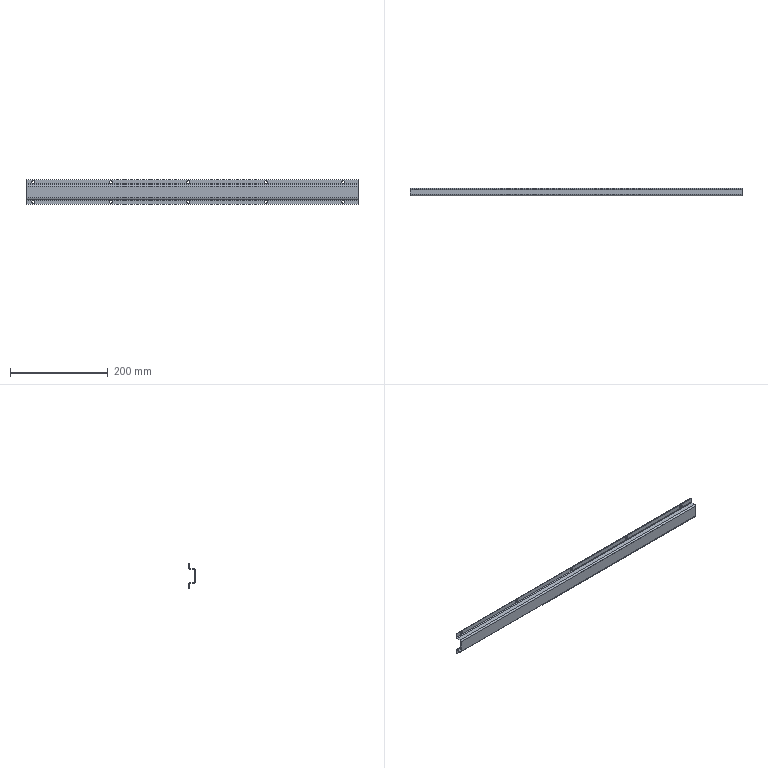Part | NX | features solid 2 | 1 solid | 42 faces | box 678 x 14.5 x 50 mm | volume 72939 mm3 | cylinder 28 | plane 14 | commonest cylinder face diameters 6 x24 3 x4
STEP:
#1=CARTESIAN_POINT('',(-1044.,518.,922.5));
#2=VERTEX_POINT('',#1);
#3=CARTESIAN_POINT('',(-1044.,519.5,922.5));
#4=VERTEX_POINT('',#3);
#5=CARTESIAN_POINT('',(-1044.,1197.996,922.5));
#6=DIRECTION('',(0.,-1.,0.));
#7=VECTOR('',#6,1000.);
#8=LINE('',#5,#7);
#9=EDGE_CURVE('',#2,#4,#8,.F.);
#10=ORIENTED_EDGE('',*,*,#9,.T.);
#11=CARTESIAN_POINT('',(-1044.,519.5,916.5));
#12=VERTEX_POINT('',#11);
#13=CARTESIAN_POINT('',(-1044.,519.5,919.5));
#14=DIRECTION('',(0.,-1.,0.));
#15=DIRECTION('',(0.,0.,-1.));
#16=AXIS2_PLACEMENT_3D('',#13,#14,#15);
#17=CIRCLE('',#16,3.);
#18=EDGE_CURVE('',#12,#4,#17,.T.);
#19=ORIENTED_EDGE('',*,*,#18,.F.);
#20=CARTESIAN_POINT('',(-1044.,518.,916.5));
#21=VERTEX_POINT('',#20);
#22=CARTESIAN_POINT('',(-1044.,1197.996,916.5));
#23=DIRECTION('',(0.,-1.,0.));
#24=VECTOR('',#23,1000.);
#25=LINE('',#22,#24);
#26=EDGE_CURVE('',#12,#21,#25,.T.);
#27=ORIENTED_EDGE('',*,*,#26,.T.);
#28=CARTESIAN_POINT('',(-1044.,518.,919.5));
#29=DIRECTION('',(0.,-1.,0.));
#30=DIRECTION('',(1.,0.,0.));
#31=AXIS2_PLACEMENT_3D('',#28,#29,#30);
#32=CIRCLE('',#31,3.);
#33=EDGE_CURVE('',#21,#2,#32,.T.);
#34=ORIENTED_EDGE('',*,*,#33,.T.);
#35=EDGE_LOOP('',(#10,#19,#27,#34));
#36=FACE_BOUND('',#35,.T.);
#37=CARTESIAN_POINT('',(-1044.,1197.996,919.5));
#38=DIRECTION('',(0.,-1.,0.));
#39=DIRECTION('',(0.,0.,-1.));
#40=AXIS2_PLACEMENT_3D('',#37,#38,#39);
#41=CYLINDRICAL_SURFACE('',#40,3.);
#42=ADVANCED_FACE('',(#36),#41,.F.);
#43=CARTESIAN_POINT('',(-1044.,518.,882.5));
#44=VERTEX_POINT('',#43);
#45=CARTESIAN_POINT('',(-1044.,519.5,882.5));
#46=VERTEX_POINT('',#45);
#47=CARTESIAN_POINT('',(-1044.,1197.996,882.5));
#48=DIRECTION('',(0.,-1.,0.));
#49=VECTOR('',#48,1000.);
#50=LINE('',#47,#49);
#51=EDGE_CURVE('',#44,#46,#50,.F.);
#52=ORIENTED_EDGE('',*,*,#51,.T.);
#53=CARTESIAN_POINT('',(-1044.,519.5,876.5));
#54=VERTEX_POINT('',#53);
#55=CARTESIAN_POINT('',(-1044.,519.5,879.5));
#56=DIRECTION('',(0.,-1.,0.));
#57=DIRECTION('',(0.,0.,-1.));
#58=AXIS2_PLACEMENT_3D('',#55,#56,#57);
#59=CIRCLE('',#58,3.);
#60=EDGE_CURVE('',#54,#46,#59,.T.);
#61=ORIENTED_EDGE('',*,*,#60,.F.);
#62=CARTESIAN_POINT('',(-1044.,518.,876.5));
#63=VERTEX_POINT('',#62);
#64=CARTESIAN_POINT('',(-1044.,1197.996,876.5));
#65=DIRECTION('',(0.,-1.,0.));
#66=VECTOR('',#65,1000.);
#67=LINE('',#64,#66);
#68=EDGE_CURVE('',#54,#63,#67,.T.);
#69=ORIENTED_EDGE('',*,*,#68,.T.);
#70=CARTESIAN_POINT('',(-1044.,518.,879.5));
#71=DIRECTION('',(0.,-1.,0.));
#72=DIRECTION('',(1.,0.,0.));
#73=AXIS2_PLACEMENT_3D('',#70,#71,#72);
#74=CIRCLE('',#73,3.);
#75=EDGE_CURVE('',#63,#44,#74,.T.);
#76=ORIENTED_EDGE('',*,*,#75,.T.);
#77=EDGE_LOOP('',(#52,#61,#69,#76));
#78=FACE_BOUND('',#77,.T.);
#79=CARTESIAN_POINT('',(-1044.,1197.996,879.5));
#80=DIRECTION('',(0.,-1.,0.));
#81=DIRECTION('',(0.,0.,-1.));
#82=AXIS2_PLACEMENT_3D('',#79,#80,#81);
#83=CYLINDRICAL_SURFACE('',#82,3.);
#84=ADVANCED_FACE('',(#78),#83,.F.);
#85=ORIENTED_EDGE('',*,*,#18,.T.);
#86=CARTESIAN_POINT('',(-1044.,519.5,919.5));
#87=DIRECTION('',(0.,-1.,0.));
#88=DIRECTION('',(0.,0.,-1.));
#89=AXIS2_PLACEMENT_3D('',#86,#87,#88);
#90=CIRCLE('',#89,3.);
#91=EDGE_CURVE('',#4,#12,#90,.T.);
#92=ORIENTED_EDGE('',*,*,#91,.T.);
#93=EDGE_LOOP('',(#85,#92));
#94=FACE_BOUND('',#93,.T.);
#95=CARTESIAN_POINT('',(-885.75,519.5,916.5));
#96=VERTEX_POINT('',#95);
#97=CARTESIAN_POINT('',(-885.75,519.5,922.5));
#98=VERTEX_POINT('',#97);
#99=CARTESIAN_POINT('',(-885.75,519.5,919.5));
#100=DIRECTION('',(0.,-1.,0.));
#101=DIRECTION('',(0.,0.,-1.));
#102=AXIS2_PLACEMENT_3D('',#99,#100,#101);
#103=CIRCLE('',#102,3.);
#104=EDGE_CURVE('',#96,#98,#103,.T.);
#105=ORIENTED_EDGE('',*,*,#104,.T.);
#106=CARTESIAN_POINT('',(-885.75,519.5,919.5));
#107=DIRECTION('',(0.,-1.,0.));
#108=DIRECTION('',(0.,0.,-1.));
#109=AXIS2_PLACEMENT_3D('',#106,#107,#108);
#110=CIRCLE('',#109,3.);
#111=EDGE_CURVE('',#98,#96,#110,.T.);
#112=ORIENTED_EDGE('',*,*,#111,.T.);
#113=EDGE_LOOP('',(#105,#112));
#114=FACE_BOUND('',#113,.T.);
#115=CARTESIAN_POINT('',(-727.5,519.5,916.5));
#116=VERTEX_POINT('',#115);
#117=CARTESIAN_POINT('',(-727.5,519.5,922.5));
#118=VERTEX_POINT('',#117);
#119=CARTESIAN_POINT('',(-727.5,519.5,919.5));
#120=DIRECTION('',(0.,-1.,0.));
#121=DIRECTION('',(0.,0.,-1.));
#122=AXIS2_PLACEMENT_3D('',#119,#120,#121);
#123=CIRCLE('',#122,3.);
#124=EDGE_CURVE('',#116,#118,#123,.T.);
#125=ORIENTED_EDGE('',*,*,#124,.T.);
#126=CARTESIAN_POINT('',(-727.5,519.5,919.5));
#127=DIRECTION('',(0.,-1.,0.));
#128=DIRECTION('',(0.,0.,-1.));
#129=AXIS2_PLACEMENT_3D('',#126,#127,#128);
#130=CIRCLE('',#129,3.);
#131=EDGE_CURVE('',#118,#116,#130,.T.);
#132=ORIENTED_EDGE('',*,*,#131,.T.);
#133=EDGE_LOOP('',(#125,#132));
#134=FACE_BOUND('',#133,.T.);
#135=CARTESIAN_POINT('',(-569.25,519.5,916.5));
#136=VERTEX_POINT('',#135);
#137=CARTESIAN_POINT('',(-569.25,519.5,922.5));
#138=VERTEX_POINT('',#137);
#139=CARTESIAN_POINT('',(-569.25,519.5,919.5));
#140=DIRECTION('',(0.,-1.,0.));
#141=DIRECTION('',(0.,0.,-1.));
#142=AXIS2_PLACEMENT_3D('',#139,#140,#141);
#143=CIRCLE('',#142,3.);
#144=EDGE_CURVE('',#136,#138,#143,.T.);
#145=ORIENTED_EDGE('',*,*,#144,.T.);
#146=CARTESIAN_POINT('',(-569.25,519.5,919.5));
#147=DIRECTION('',(0.,-1.,0.));
#148=DIRECTION('',(0.,0.,-1.));
#149=AXIS2_PLACEMENT_3D('',#146,#147,#148);
#150=CIRCLE('',#149,3.);
#151=EDGE_CURVE('',#138,#136,#150,.T.);
#152=ORIENTED_EDGE('',*,*,#151,.T.);
#153=EDGE_LOOP('',(#145,#152));
#154=FACE_BOUND('',#153,.T.);
#155=CARTESIAN_POINT('',(-411.,519.5,916.5));
#156=VERTEX_POINT('',#155);
#157=CARTESIAN_POINT('',(-411.,519.5,922.5));
#158=VERTEX_POINT('',#157);
#159=CARTESIAN_POINT('',(-411.,519.5,919.5));
#160=DIRECTION('',(0.,-1.,0.));
#161=DIRECTION('',(0.,0.,-1.));
#162=AXIS2_PLACEMENT_3D('',#159,#160,#161);
#163=CIRCLE('',#162,3.);
#164=EDGE_CURVE('',#156,#158,#163,.T.);
#165=ORIENTED_EDGE('',*,*,#164,.T.);
#166=CARTESIAN_POINT('',(-411.,519.5,919.5));
#167=DIRECTION('',(0.,-1.,0.));
#168=DIRECTION('',(0.,0.,-1.));
#169=AXIS2_PLACEMENT_3D('',#166,#167,#168);
#170=CIRCLE('',#169,3.);
#171=EDGE_CURVE('',#158,#156,#170,.T.);
#172=ORIENTED_EDGE('',*,*,#171,.T.);
#173=EDGE_LOOP('',(#165,#172));
#174=FACE_BOUND('',#173,.T.);
#175=CARTESIAN_POINT('',(-1059.,519.5,916.));
#176=VERTEX_POINT('',#175);
#177=CARTESIAN_POINT('',(-1059.,519.5,924.5));
#178=VERTEX_POINT('',#177);
#179=CARTESIAN_POINT('',(-1059.,519.5,914.5));
#180=DIRECTION('',(0.,0.,1.));
#181=VECTOR('',#180,1000.);
#182=LINE('',#179,#181);
#183=EDGE_CURVE('',#176,#178,#182,.T.);
#184=ORIENTED_EDGE('',*,*,#183,.T.);
#185=CARTESIAN_POINT('',(-381.,519.5,924.5));
#186=VERTEX_POINT('',#185);
#187=CARTESIAN_POINT('',(-381.,519.5,924.5));
#188=DIRECTION('',(-1.,0.,0.));
#189=VECTOR('',#188,1000.);
#190=LINE('',#187,#189);
#191=EDGE_CURVE('',#186,#178,#190,.T.);
#192=ORIENTED_EDGE('',*,*,#191,.F.);
#193=CARTESIAN_POINT('',(-381.,519.5,916.));
#194=VERTEX_POINT('',#193);
#195=CARTESIAN_POINT('',(-381.,519.5,914.5));
#196=DIRECTION('',(0.,0.,1.));
#197=VECTOR('',#196,1000.);
#198=LINE('',#195,#197);
#199=EDGE_CURVE('',#194,#186,#198,.T.);
#200=ORIENTED_EDGE('',*,*,#199,.F.);
#201=CARTESIAN_POINT('',(-381.,519.5,916.));
#202=DIRECTION('',(-1.,0.,0.));
#203=VECTOR('',#202,1000.);
#204=LINE('',#201,#203);
#205=EDGE_CURVE('',#194,#176,#204,.T.);
#206=ORIENTED_EDGE('',*,*,#205,.T.);
#207=EDGE_LOOP('',(#184,#192,#200,#206));
#208=FACE_BOUND('',#207,.T.);
#209=CARTESIAN_POINT('',(-381.,519.5,914.5));
#210=DIRECTION('',(0.,-1.,0.));
#211=DIRECTION('',(-1.,0.,0.));
#212=AXIS2_PLACEMENT_3D('',#209,#210,#211);
#213=PLANE('',#212);
#214=ADVANCED_FACE('',(#94,#114,#134,#154,#174,#208),#213,.F.);
#215=CARTESIAN_POINT('',(-1059.,516.5,913.));
#216=VERTEX_POINT('',#215);
#217=CARTESIAN_POINT('',(-1059.,516.5,916.));
#218=DIRECTION('',(1.,0.,0.));
#219=DIRECTION('',(0.,0.,1.));
#220=AXIS2_PLACEMENT_3D('',#217,#218,#219);
#221=CIRCLE('',#220,3.);
#222=EDGE_CURVE('',#216,#176,#221,.T.);
#223=ORIENTED_EDGE('',*,*,#222,.T.);
#224=ORIENTED_EDGE('',*,*,#205,.F.);
#225=CARTESIAN_POINT('',(-381.,516.5,913.));
#226=VERTEX_POINT('',#225);
#227=CARTESIAN_POINT('',(-381.,516.5,916.));
#228=DIRECTION('',(1.,0.,0.));
#229=DIRECTION('',(0.,0.,1.));
#230=AXIS2_PLACEMENT_3D('',#227,#228,#229);
#231=CIRCLE('',#230,3.);
#232=EDGE_CURVE('',#226,#194,#231,.T.);
#233=ORIENTED_EDGE('',*,*,#232,.F.);
#234=CARTESIAN_POINT('',(-381.,516.5,913.));
#235=DIRECTION('',(-1.,0.,0.));
#236=VECTOR('',#235,1000.);
#237=LINE('',#234,#236);
#238=EDGE_CURVE('',#226,#216,#237,.T.);
#239=ORIENTED_EDGE('',*,*,#238,.T.);
#240=EDGE_LOOP('',(#223,#224,#233,#239));
#241=FACE_BOUND('',#240,.T.);
#242=CARTESIAN_POINT('',(-381.,516.5,916.));
#243=DIRECTION('',(-1.,0.,0.));
#244=DIRECTION('',(0.,0.,1.));
#245=AXIS2_PLACEMENT_3D('',#242,#243,#244);
#246=CYLINDRICAL_SURFACE('',#245,3.);
#247=ADVANCED_FACE('',(#241),#246,.T.);
#248=CARTESIAN_POINT('',(-1059.,508.,913.));
#249=VERTEX_POINT('',#248);
#250=CARTESIAN_POINT('',(-1059.,505.,913.));
#251=DIRECTION('',(0.,1.,0.));
#252=VECTOR('',#251,1000.);
#253=LINE('',#250,#252);
#254=EDGE_CURVE('',#249,#216,#253,.T.);
#255=ORIENTED_EDGE('',*,*,#254,.T.);
#256=ORIENTED_EDGE('',*,*,#238,.F.);
#257=CARTESIAN_POINT('',(-381.,508.,913.));
#258=VERTEX_POINT('',#257);
#259=CARTESIAN_POINT('',(-381.,505.,913.));
#260=DIRECTION('',(0.,1.,0.));
#261=VECTOR('',#260,1000.);
#262=LINE('',#259,#261);
#263=EDGE_CURVE('',#258,#226,#262,.T.);
#264=ORIENTED_EDGE('',*,*,#263,.F.);
#265=CARTESIAN_POINT('',(-381.,508.,913.));
#266=DIRECTION('',(-1.,0.,0.));
#267=VECTOR('',#266,1000.);
#268=LINE('',#265,#267);
#269=EDGE_CURVE('',#258,#249,#268,.T.);
#270=ORIENTED_EDGE('',*,*,#269,.T.);
#271=EDGE_LOOP('',(#255,#256,#264,#270));
#272=FACE_BOUND('',#271,.T.);
#273=CARTESIAN_POINT('',(-381.,505.,913.));
#274=DIRECTION('',(0.,0.,1.));
#275=DIRECTION('',(0.,-1.,0.));
#276=AXIS2_PLACEMENT_3D('',#273,#274,#275);
#277=PLANE('',#276);
#278=ADVANCED_FACE('',(#272),#277,.F.);
#279=CARTESIAN_POINT('',(-1059.,506.5,911.5));
#280=VERTEX_POINT('',#279);
#281=CARTESIAN_POINT('',(-1059.,508.,911.5));
#282=DIRECTION('',(-1.,0.,0.));
#283=DIRECTION('',(0.,0.,1.));
#284=AXIS2_PLACEMENT_3D('',#281,#282,#283);
#285=CIRCLE('',#284,1.5);
#286=EDGE_CURVE('',#280,#249,#285,.T.);
#287=ORIENTED_EDGE('',*,*,#286,.T.);
#288=ORIENTED_EDGE('',*,*,#269,.F.);
#289=CARTESIAN_POINT('',(-381.,506.5,911.5));
#290=VERTEX_POINT('',#289);
#291=CARTESIAN_POINT('',(-381.,508.,911.5));
#292=DIRECTION('',(-1.,0.,0.));
#293=DIRECTION('',(0.,0.,1.));
#294=AXIS2_PLACEMENT_3D('',#291,#292,#293);
#295=CIRCLE('',#294,1.5);
#296=EDGE_CURVE('',#290,#258,#295,.T.);
#297=ORIENTED_EDGE('',*,*,#296,.F.);
#298=CARTESIAN_POINT('',(-381.,506.5,911.5));
#299=DIRECTION('',(-1.,0.,0.));
#300=VECTOR('',#299,1000.);
#301=LINE('',#298,#300);
#302=EDGE_CURVE('',#290,#280,#301,.T.);
#303=ORIENTED_EDGE('',*,*,#302,.T.);
#304=EDGE_LOOP('',(#287,#288,#297,#303));
#305=FACE_BOUND('',#304,.T.);
#306=CARTESIAN_POINT('',(-381.,508.,911.5));
#307=DIRECTION('',(-1.,0.,0.));
#308=DIRECTION('',(0.,0.,1.));
#309=AXIS2_PLACEMENT_3D('',#306,#307,#308);
#310=CYLINDRICAL_SURFACE('',#309,1.5);
#311=ADVANCED_FACE('',(#305),#310,.F.);
#312=CARTESIAN_POINT('',(-1059.,506.5,887.5));
#313=VERTEX_POINT('',#312);
#314=CARTESIAN_POINT('',(-1059.,506.5,884.5));
#315=DIRECTION('',(0.,0.,1.));
#316=VECTOR('',#315,1000.);
#317=LINE('',#314,#316);
#318=EDGE_CURVE('',#313,#280,#317,.T.);
#319=ORIENTED_EDGE('',*,*,#318,.T.);
#320=ORIENTED_EDGE('',*,*,#302,.F.);
#321=CARTESIAN_POINT('',(-381.,506.5,887.5));
#322=VERTEX_POINT('',#321);
#323=CARTESIAN_POINT('',(-381.,506.5,884.5));
#324=DIRECTION('',(0.,0.,1.));
#325=VECTOR('',#324,1000.);
#326=LINE('',#323,#325);
#327=EDGE_CURVE('',#322,#290,#326,.T.);
#328=ORIENTED_EDGE('',*,*,#327,.F.);
#329=CARTESIAN_POINT('',(-381.,506.5,887.5));
#330=DIRECTION('',(-1.,0.,0.));
#331=VECTOR('',#330,1000.);
#332=LINE('',#329,#331);
#333=EDGE_CURVE('',#322,#313,#332,.T.);
#334=ORIENTED_EDGE('',*,*,#333,.T.);
#335=EDGE_LOOP('',(#319,#320,#328,#334));
#336=FACE_BOUND('',#335,.T.);
#337=CARTESIAN_POINT('',(-381.,506.5,884.5));
#338=DIRECTION('',(0.,-1.,0.));
#339=DIRECTION('',(-1.,0.,0.));
#340=AXIS2_PLACEMENT_3D('',#337,#338,#339);
#341=PLANE('',#340);
#342=ADVANCED_FACE('',(#336),#341,.F.);
#343=CARTESIAN_POINT('',(-1059.,508.,886.));
#344=VERTEX_POINT('',#343);
#345=CARTESIAN_POINT('',(-1059.,508.,887.5));
#346=DIRECTION('',(-1.,0.,0.));
#347=DIRECTION('',(0.,0.,1.));
#348=AXIS2_PLACEMENT_3D('',#345,#346,#347);
#349=CIRCLE('',#348,1.5);
#350=EDGE_CURVE('',#344,#313,#349,.T.);
#351=ORIENTED_EDGE('',*,*,#350,.T.);
#352=ORIENTED_EDGE('',*,*,#333,.F.);
#353=CARTESIAN_POINT('',(-381.,508.,886.));
#354=VERTEX_POINT('',#353);
#355=CARTESIAN_POINT('',(-381.,508.,887.5));
#356=DIRECTION('',(-1.,0.,0.));
#357=DIRECTION('',(0.,0.,1.));
#358=AXIS2_PLACEMENT_3D('',#355,#356,#357);
#359=CIRCLE('',#358,1.5);
#360=EDGE_CURVE('',#354,#322,#359,.T.);
#361=ORIENTED_EDGE('',*,*,#360,.F.);
#362=CARTESIAN_POINT('',(-381.,508.,886.));
#363=DIRECTION('',(-1.,0.,0.));
#364=VECTOR('',#363,1000.);
#365=LINE('',#362,#364);
#366=EDGE_CURVE('',#354,#344,#365,.T.);
#367=ORIENTED_EDGE('',*,*,#366,.T.);
#368=EDGE_LOOP('',(#351,#352,#361,#367));
#369=FACE_BOUND('',#368,.T.);
#370=CARTESIAN_POINT('',(-381.,508.,887.5));
#371=DIRECTION('',(-1.,0.,0.));
#372=DIRECTION('',(0.,0.,1.));
#373=AXIS2_PLACEMENT_3D('',#370,#371,#372);
#374=CYLINDRICAL_SURFACE('',#373,1.5);
#375=ADVANCED_FACE('',(#369),#374,.F.);
#376=CARTESIAN_POINT('',(-1059.,516.5,886.));
#377=VERTEX_POINT('',#376);
#378=CARTESIAN_POINT('',(-1059.,518.,886.));
#379=DIRECTION('',(0.,-1.,0.));
#380=VECTOR('',#379,1000.);
#381=LINE('',#378,#380);
#382=EDGE_CURVE('',#377,#344,#381,.T.);
#383=ORIENTED_EDGE('',*,*,#382,.T.);
#384=ORIENTED_EDGE('',*,*,#366,.F.);
#385=CARTESIAN_POINT('',(-381.,516.5,886.));
#386=VERTEX_POINT('',#385);
#387=CARTESIAN_POINT('',(-381.,518.,886.));
#388=DIRECTION('',(0.,-1.,0.));
#389=VECTOR('',#388,1000.);
#390=LINE('',#387,#389);
#391=EDGE_CURVE('',#386,#354,#390,.T.);
#392=ORIENTED_EDGE('',*,*,#391,.F.);
#393=CARTESIAN_POINT('',(-381.,516.5,886.));
#394=DIRECTION('',(-1.,0.,0.));
#395=VECTOR('',#394,1000.);
#396=LINE('',#393,#395);
#397=EDGE_CURVE('',#386,#377,#396,.T.);
#398=ORIENTED_EDGE('',*,*,#397,.T.);
#399=EDGE_LOOP('',(#383,#384,#392,#398));
#400=FACE_BOUND('',#399,.T.);
#401=CARTESIAN_POINT('',(-381.,518.,886.));
#402=DIRECTION('',(0.,0.,-1.));
#403=DIRECTION('',(0.,-1.,0.));
#404=AXIS2_PLACEMENT_3D('',#401,#402,#403);
#405=PLANE('',#404);
#406=ADVANCED_FACE('',(#400),#405,.F.);
#407=CARTESIAN_POINT('',(-1059.,519.5,883.));
#408=VERTEX_POINT('',#407);
#409=CARTESIAN_POINT('',(-1059.,516.5,883.));
#410=DIRECTION('',(1.,0.,0.));
#411=DIRECTION('',(0.,0.,1.));
#412=AXIS2_PLACEMENT_3D('',#409,#410,#411);
#413=CIRCLE('',#412,3.);
#414=EDGE_CURVE('',#408,#377,#413,.T.);
#415=ORIENTED_EDGE('',*,*,#414,.T.);
#416=ORIENTED_EDGE('',*,*,#397,.F.);
#417=CARTESIAN_POINT('',(-381.,519.5,883.));
#418=VERTEX_POINT('',#417);
#419=CARTESIAN_POINT('',(-381.,516.5,883.));
#420=DIRECTION('',(1.,0.,0.));
#421=DIRECTION('',(0.,0.,1.));
#422=AXIS2_PLACEMENT_3D('',#419,#420,#421);
#423=CIRCLE('',#422,3.);
#424=EDGE_CURVE('',#418,#386,#423,.T.);
#425=ORIENTED_EDGE('',*,*,#424,.F.);
#426=CARTESIAN_POINT('',(-381.,519.5,883.));
#427=DIRECTION('',(-1.,0.,0.));
#428=VECTOR('',#427,1000.);
#429=LINE('',#426,#428);
#430=EDGE_CURVE('',#418,#408,#429,.T.);
#431=ORIENTED_EDGE('',*,*,#430,.T.);
#432=EDGE_LOOP('',(#415,#416,#425,#431));
#433=FACE_BOUND('',#432,.T.);
#434=CARTESIAN_POINT('',(-381.,516.5,883.));
#435=DIRECTION('',(-1.,0.,0.));
#436=DIRECTION('',(0.,0.,1.));
#437=AXIS2_PLACEMENT_3D('',#434,#435,#436);
#438=CYLINDRICAL_SURFACE('',#437,3.);
#439=ADVANCED_FACE('',(#433),#438,.T.);
#440=ORIENTED_EDGE('',*,*,#60,.T.);
#441=CARTESIAN_POINT('',(-1044.,519.5,879.5));
#442=DIRECTION('',(0.,-1.,0.));
#443=DIRECTION('',(0.,0.,-1.));
#444=AXIS2_PLACEMENT_3D('',#441,#442,#443);
#445=CIRCLE('',#444,3.);
#446=EDGE_CURVE('',#46,#54,#445,.T.);
#447=ORIENTED_EDGE('',*,*,#446,.T.);
#448=EDGE_LOOP('',(#440,#447));
#449=FACE_BOUND('',#448,.T.);
#450=CARTESIAN_POINT('',(-885.75,519.5,876.5));
#451=VERTEX_POINT('',#450);
#452=CARTESIAN_POINT('',(-885.75,519.5,882.5));
#453=VERTEX_POINT('',#452);
#454=CARTESIAN_POINT('',(-885.75,519.5,879.5));
#455=DIRECTION('',(0.,-1.,0.));
#456=DIRECTION('',(0.,0.,-1.));
#457=AXIS2_PLACEMENT_3D('',#454,#455,#456);
#458=CIRCLE('',#457,3.);
#459=EDGE_CURVE('',#451,#453,#458,.T.);
#460=ORIENTED_EDGE('',*,*,#459,.T.);
#461=CARTESIAN_POINT('',(-885.75,519.5,879.5));
#462=DIRECTION('',(0.,-1.,0.));
#463=DIRECTION('',(0.,0.,-1.));
#464=AXIS2_PLACEMENT_3D('',#461,#462,#463);
#465=CIRCLE('',#464,3.);
#466=EDGE_CURVE('',#453,#451,#465,.T.);
#467=ORIENTED_EDGE('',*,*,#466,.T.);
#468=EDGE_LOOP('',(#460,#467));
#469=FACE_BOUND('',#468,.T.);
#470=CARTESIAN_POINT('',(-727.5,519.5,876.5));
#471=VERTEX_POINT('',#470);
#472=CARTESIAN_POINT('',(-727.5,519.5,882.5));
#473=VERTEX_POINT('',#472);
#474=CARTESIAN_POINT('',(-727.5,519.5,879.5));
#475=DIRECTION('',(0.,-1.,0.));
#476=DIRECTION('',(0.,0.,-1.));
#477=AXIS2_PLACEMENT_3D('',#474,#475,#476);
#478=CIRCLE('',#477,3.);
#479=EDGE_CURVE('',#471,#473,#478,.T.);
#480=ORIENTED_EDGE('',*,*,#479,.T.);
#481=CARTESIAN_POINT('',(-727.5,519.5,879.5));
#482=DIRECTION('',(0.,-1.,0.));
#483=DIRECTION('',(0.,0.,-1.));
#484=AXIS2_PLACEMENT_3D('',#481,#482,#483);
#485=CIRCLE('',#484,3.);
#486=EDGE_CURVE('',#473,#471,#485,.T.);
#487=ORIENTED_EDGE('',*,*,#486,.T.);
#488=EDGE_LOOP('',(#480,#487));
#489=FACE_BOUND('',#488,.T.);
#490=CARTESIAN_POINT('',(-569.25,519.5,876.5));
#491=VERTEX_POINT('',#490);
#492=CARTESIAN_POINT('',(-569.25,519.5,882.5));
#493=VERTEX_POINT('',#492);
#494=CARTESIAN_POINT('',(-569.25,519.5,879.5));
#495=DIRECTION('',(0.,-1.,0.));
#496=DIRECTION('',(0.,0.,-1.));
#497=AXIS2_PLACEMENT_3D('',#494,#495,#496);
#498=CIRCLE('',#497,3.);
#499=EDGE_CURVE('',#491,#493,#498,.T.);
#500=ORIENTED_EDGE('',*,*,#499,.T.);
#501=CARTESIAN_POINT('',(-569.25,519.5,879.5));
#502=DIRECTION('',(0.,-1.,0.));
#503=DIRECTION('',(0.,0.,-1.));
#504=AXIS2_PLACEMENT_3D('',#501,#502,#503);
#505=CIRCLE('',#504,3.);
#506=EDGE_CURVE('',#493,#491,#505,.T.);
#507=ORIENTED_EDGE('',*,*,#506,.T.);
#508=EDGE_LOOP('',(#500,#507));
#509=FACE_BOUND('',#508,.T.);
#510=CARTESIAN_POINT('',(-411.,519.5,876.5));
#511=VERTEX_POINT('',#510);
#512=CARTESIAN_POINT('',(-411.,519.5,882.5));
#513=VERTEX_POINT('',#512);
#514=CARTESIAN_POINT('',(-411.,519.5,879.5));
#515=DIRECTION('',(0.,-1.,0.));
#516=DIRECTION('',(0.,0.,-1.));
#517=AXIS2_PLACEMENT_3D('',#514,#515,#516);
#518=CIRCLE('',#517,3.);
#519=EDGE_CURVE('',#511,#513,#518,.T.);
#520=ORIENTED_EDGE('',*,*,#519,.T.);
#521=CARTESIAN_POINT('',(-411.,519.5,879.5));
#522=DIRECTION('',(0.,-1.,0.));
#523=DIRECTION('',(0.,0.,-1.));
#524=AXIS2_PLACEMENT_3D('',#521,#522,#523);
#525=CIRCLE('',#524,3.);
#526=EDGE_CURVE('',#513,#511,#525,.T.);
#527=ORIENTED_EDGE('',*,*,#526,.T.);
#528=EDGE_LOOP('',(#520,#527));
#529=FACE_BOUND('',#528,.T.);
#530=CARTESIAN_POINT('',(-1059.,519.5,874.5));
#531=VERTEX_POINT('',#530);
#532=CARTESIAN_POINT('',(-1059.,519.5,874.5));
#533=DIRECTION('',(0.,0.,1.));
#534=VECTOR('',#533,1000.);
#535=LINE('',#532,#534);
#536=EDGE_CURVE('',#531,#408,#535,.T.);
#537=ORIENTED_EDGE('',*,*,#536,.T.);
#538=ORIENTED_EDGE('',*,*,#430,.F.);
#539=CARTESIAN_POINT('',(-381.,519.5,874.5));
#540=VERTEX_POINT('',#539);
#541=CARTESIAN_POINT('',(-381.,519.5,874.5));
#542=DIRECTION('',(0.,0.,1.));
#543=VECTOR('',#542,1000.);
#544=LINE('',#541,#543);
#545=EDGE_CURVE('',#540,#418,#544,.T.);
#546=ORIENTED_EDGE('',*,*,#545,.F.);
#547=CARTESIAN_POINT('',(-381.,519.5,874.5));
#548=DIRECTION('',(-1.,0.,0.));
#549=VECTOR('',#548,1000.);
#550=LINE('',#547,#549);
#551=EDGE_CURVE('',#540,#531,#550,.T.);
#552=ORIENTED_EDGE('',*,*,#551,.T.);
#553=EDGE_LOOP('',(#537,#538,#546,#552));
#554=FACE_BOUND('',#553,.T.);
#555=CARTESIAN_POINT('',(-381.,519.5,874.5));
#556=DIRECTION('',(0.,-1.,0.));
#557=DIRECTION('',(-1.,0.,0.));
#558=AXIS2_PLACEMENT_3D('',#555,#556,#557);
#559=PLANE('',#558);
#560=ADVANCED_FACE('',(#449,#469,#489,#509,#529,#554),#559,.F.);
#561=ORIENTED_EDGE('',*,*,#33,.F.);
#562=CARTESIAN_POINT('',(-1044.,518.,919.5));
#563=DIRECTION('',(0.,-1.,0.));
#564=DIRECTION('',(1.,0.,0.));
#565=AXIS2_PLACEMENT_3D('',#562,#563,#564);
#566=CIRCLE('',#565,3.);
#567=EDGE_CURVE('',#2,#21,#566,.T.);
#568=ORIENTED_EDGE('',*,*,#567,.F.);
#569=EDGE_LOOP('',(#561,#568));
#570=FACE_BOUND('',#569,.T.);
#571=CARTESIAN_POINT('',(-885.75,518.,916.5));
#572=VERTEX_POINT('',#571);
#573=CARTESIAN_POINT('',(-885.75,518.,922.5));
#574=VERTEX_POINT('',#573);
#575=CARTESIAN_POINT('',(-885.75,518.,919.5));
#576=DIRECTION('',(0.,-1.,0.));
#577=DIRECTION('',(1.,0.,0.));
#578=AXIS2_PLACEMENT_3D('',#575,#576,#577);
#579=CIRCLE('',#578,3.);
#580=EDGE_CURVE('',#572,#574,#579,.T.);
#581=ORIENTED_EDGE('',*,*,#580,.F.);
#582=CARTESIAN_POINT('',(-885.75,518.,919.5));
#583=DIRECTION('',(0.,-1.,0.));
#584=DIRECTION('',(1.,0.,0.));
#585=AXIS2_PLACEMENT_3D('',#582,#583,#584);
#586=CIRCLE('',#585,3.);
#587=EDGE_CURVE('',#574,#572,#586,.T.);
#588=ORIENTED_EDGE('',*,*,#587,.F.);
#589=EDGE_LOOP('',(#581,#588));
#590=FACE_BOUND('',#589,.T.);
#591=CARTESIAN_POINT('',(-727.5,518.,916.5));
#592=VERTEX_POINT('',#591);
#593=CARTESIAN_POINT('',(-727.5,518.,922.5));
#594=VERTEX_POINT('',#593);
#595=CARTESIAN_POINT('',(-727.5,518.,919.5));
#596=DIRECTION('',(0.,-1.,0.));
#597=DIRECTION('',(1.,0.,0.));
#598=AXIS2_PLACEMENT_3D('',#595,#596,#597);
#599=CIRCLE('',#598,3.);
#600=EDGE_CURVE('',#592,#594,#599,.T.);
#601=ORIENTED_EDGE('',*,*,#600,.F.);
#602=CARTESIAN_POINT('',(-727.5,518.,919.5));
#603=DIRECTION('',(0.,-1.,0.));
#604=DIRECTION('',(1.,0.,0.));
#605=AXIS2_PLACEMENT_3D('',#602,#603,#604);
#606=CIRCLE('',#605,3.);
#607=EDGE_CURVE('',#594,#592,#606,.T.);
#608=ORIENTED_EDGE('',*,*,#607,.F.);
#609=EDGE_LOOP('',(#601,#608));
#610=FACE_BOUND('',#609,.T.);
#611=CARTESIAN_POINT('',(-569.25,518.,916.5));
#612=VERTEX_POINT('',#611);
#613=CARTESIAN_POINT('',(-569.25,518.,922.5));
#614=VERTEX_POINT('',#613);
#615=CARTESIAN_POINT('',(-569.25,518.,919.5));
#616=DIRECTION('',(0.,-1.,0.));
#617=DIRECTION('',(1.,0.,0.));
#618=AXIS2_PLACEMENT_3D('',#615,#616,#617);
#619=CIRCLE('',#618,3.);
#620=EDGE_CURVE('',#612,#614,#619,.T.);
#621=ORIENTED_EDGE('',*,*,#620,.F.);
#622=CARTESIAN_POINT('',(-569.25,518.,919.5));
#623=DIRECTION('',(0.,-1.,0.));
#624=DIRECTION('',(1.,0.,0.));
#625=AXIS2_PLACEMENT_3D('',#622,#623,#624);
#626=CIRCLE('',#625,3.);
#627=EDGE_CURVE('',#614,#612,#626,.T.);
#628=ORIENTED_EDGE('',*,*,#627,.F.);
#629=EDGE_LOOP('',(#621,#628));
#630=FACE_BOUND('',#629,.T.);
#631=CARTESIAN_POINT('',(-411.,518.,916.5));
#632=VERTEX_POINT('',#631);
#633=CARTESIAN_POINT('',(-411.,518.,922.5));
#634=VERTEX_POINT('',#633);
#635=CARTESIAN_POINT('',(-411.,518.,919.5));
#636=DIRECTION('',(0.,-1.,0.));
#637=DIRECTION('',(1.,0.,0.));
#638=AXIS2_PLACEMENT_3D('',#635,#636,#637);
#639=CIRCLE('',#638,3.);
#640=EDGE_CURVE('',#632,#634,#639,.T.);
#641=ORIENTED_EDGE('',*,*,#640,.F.);
#642=CARTESIAN_POINT('',(-411.,518.,919.5));
#643=DIRECTION('',(0.,-1.,0.));
#644=DIRECTION('',(1.,0.,0.));
#645=AXIS2_PLACEMENT_3D('',#642,#643,#644);
#646=CIRCLE('',#645,3.);
#647=EDGE_CURVE('',#634,#632,#646,.T.);
#648=ORIENTED_EDGE('',*,*,#647,.F.);
#649=EDGE_LOOP('',(#641,#648));
#650=FACE_BOUND('',#649,.T.);
#651=CARTESIAN_POINT('',(-1059.,518.,916.));
#652=VERTEX_POINT('',#651);
#653=CARTESIAN_POINT('',(-1059.,518.,924.5));
#654=VERTEX_POINT('',#653);
#655=CARTESIAN_POINT('',(-1059.,518.,914.5));
#656=DIRECTION('',(0.,0.,1.));
#657=VECTOR('',#656,1000.);
#658=LINE('',#655,#657);
#659=EDGE_CURVE('',#652,#654,#658,.T.);
#660=ORIENTED_EDGE('',*,*,#659,.F.);
#661=CARTESIAN_POINT('',(-381.,518.,916.));
#662=VERTEX_POINT('',#661);
#663=CARTESIAN_POINT('',(-381.,518.,916.));
#664=DIRECTION('',(-1.,0.,0.));
#665=VECTOR('',#664,1000.);
#666=LINE('',#663,#665);
#667=EDGE_CURVE('',#662,#652,#666,.T.);
#668=ORIENTED_EDGE('',*,*,#667,.F.);
#669=CARTESIAN_POINT('',(-381.,518.,924.5));
#670=VERTEX_POINT('',#669);
#671=CARTESIAN_POINT('',(-381.,518.,914.5));
#672=DIRECTION('',(0.,0.,1.));
#673=VECTOR('',#672,1000.);
#674=LINE('',#671,#673);
#675=EDGE_CURVE('',#662,#670,#674,.T.);
#676=ORIENTED_EDGE('',*,*,#675,.T.);
#677=CARTESIAN_POINT('',(-381.,518.,924.5));
#678=DIRECTION('',(-1.,0.,0.));
#679=VECTOR('',#678,1000.);
#680=LINE('',#677,#679);
#681=EDGE_CURVE('',#670,#654,#680,.T.);
#682=ORIENTED_EDGE('',*,*,#681,.T.);
#683=EDGE_LOOP('',(#660,#668,#676,#682));
#684=FACE_BOUND('',#683,.T.);
#685=CARTESIAN_POINT('',(-381.,518.,914.5));
#686=DIRECTION('',(0.,-1.,0.));
#687=DIRECTION('',(-1.,0.,0.));
#688=AXIS2_PLACEMENT_3D('',#685,#686,#687);
#689=PLANE('',#688);
#690=ADVANCED_FACE('',(#570,#590,#610,#630,#650,#684),#689,.T.);
#691=CARTESIAN_POINT('',(-1059.,516.5,914.5));
#692=VERTEX_POINT('',#691);
#693=CARTESIAN_POINT('',(-1059.,516.5,916.));
#694=DIRECTION('',(1.,0.,0.));
#695=DIRECTION('',(0.,0.,1.));
#696=AXIS2_PLACEMENT_3D('',#693,#694,#695);
#697=CIRCLE('',#696,1.5);
#698=EDGE_CURVE('',#692,#652,#697,.T.);
#699=ORIENTED_EDGE('',*,*,#698,.F.);
#700=CARTESIAN_POINT('',(-381.,516.5,914.5));
#701=VERTEX_POINT('',#700);
#702=CARTESIAN_POINT('',(-381.,516.5,914.5));
#703=DIRECTION('',(-1.,0.,0.));
#704=VECTOR('',#703,1000.);
#705=LINE('',#702,#704);
#706=EDGE_CURVE('',#701,#692,#705,.T.);
#707=ORIENTED_EDGE('',*,*,#706,.F.);
#708=CARTESIAN_POINT('',(-381.,516.5,916.));
#709=DIRECTION('',(1.,0.,0.));
#710=DIRECTION('',(0.,0.,1.));
#711=AXIS2_PLACEMENT_3D('',#708,#709,#710);
#712=CIRCLE('',#711,1.5);
#713=EDGE_CURVE('',#701,#662,#712,.T.);
#714=ORIENTED_EDGE('',*,*,#713,.T.);
#715=ORIENTED_EDGE('',*,*,#667,.T.);
#716=EDGE_LOOP('',(#699,#707,#714,#715));
#717=FACE_BOUND('',#716,.T.);
#718=CARTESIAN_POINT('',(-381.,516.5,916.));
#719=DIRECTION('',(-1.,0.,0.));
#720=DIRECTION('',(0.,0.,1.));
#721=AXIS2_PLACEMENT_3D('',#718,#719,#720);
#722=CYLINDRICAL_SURFACE('',#721,1.5);
#723=ADVANCED_FACE('',(#717),#722,.F.);
#724=CARTESIAN_POINT('',(-1059.,508.,914.5));
#725=VERTEX_POINT('',#724);
#726=CARTESIAN_POINT('',(-1059.,505.,914.5));
#727=DIRECTION('',(0.,1.,0.));
#728=VECTOR('',#727,1000.);
#729=LINE('',#726,#728);
#730=EDGE_CURVE('',#725,#692,#729,.T.);
#731=ORIENTED_EDGE('',*,*,#730,.F.);
#732=CARTESIAN_POINT('',(-381.,508.,914.5));
#733=VERTEX_POINT('',#732);
#734=CARTESIAN_POINT('',(-381.,508.,914.5));
#735=DIRECTION('',(-1.,0.,0.));
#736=VECTOR('',#735,1000.);
#737=LINE('',#734,#736);
#738=EDGE_CURVE('',#733,#725,#737,.T.);
#739=ORIENTED_EDGE('',*,*,#738,.F.);
#740=CARTESIAN_POINT('',(-381.,505.,914.5));
#741=DIRECTION('',(0.,1.,0.));
#742=VECTOR('',#741,1000.);
#743=LINE('',#740,#742);
#744=EDGE_CURVE('',#733,#701,#743,.T.);
#745=ORIENTED_EDGE('',*,*,#744,.T.);
#746=ORIENTED_EDGE('',*,*,#706,.T.);
#747=EDGE_LOOP('',(#731,#739,#745,#746));
#748=FACE_BOUND('',#747,.T.);
#749=CARTESIAN_POINT('',(-381.,505.,914.5));
#750=DIRECTION('',(0.,0.,1.));
#751=DIRECTION('',(0.,-1.,0.));
#752=AXIS2_PLACEMENT_3D('',#749,#750,#751);
#753=PLANE('',#752);
#754=ADVANCED_FACE('',(#748),#753,.T.);
#755=CARTESIAN_POINT('',(-1059.,505.,911.5));
#756=VERTEX_POINT('',#755);
#757=CARTESIAN_POINT('',(-1059.,508.,911.5));
#758=DIRECTION('',(-1.,0.,0.));
#759=DIRECTION('',(0.,0.,-1.));
#760=AXIS2_PLACEMENT_3D('',#757,#758,#759);
#761=CIRCLE('',#760,3.);
#762=EDGE_CURVE('',#756,#725,#761,.T.);
#763=ORIENTED_EDGE('',*,*,#762,.F.);
#764=CARTESIAN_POINT('',(-381.,505.,911.5));
#765=VERTEX_POINT('',#764);
#766=CARTESIAN_POINT('',(-381.,505.,911.5));
#767=DIRECTION('',(-1.,0.,0.));
#768=VECTOR('',#767,1000.);
#769=LINE('',#766,#768);
#770=EDGE_CURVE('',#765,#756,#769,.T.);
#771=ORIENTED_EDGE('',*,*,#770,.F.);
#772=CARTESIAN_POINT('',(-381.,508.,911.5));
#773=DIRECTION('',(-1.,0.,0.));
#774=DIRECTION('',(0.,0.,-1.));
#775=AXIS2_PLACEMENT_3D('',#772,#773,#774);
#776=CIRCLE('',#775,3.);
#777=EDGE_CURVE('',#765,#733,#776,.T.);
#778=ORIENTED_EDGE('',*,*,#777,.T.);
#779=ORIENTED_EDGE('',*,*,#738,.T.);
#780=EDGE_LOOP('',(#763,#771,#778,#779));
#781=FACE_BOUND('',#780,.T.);
#782=CARTESIAN_POINT('',(-381.,508.,911.5));
#783=DIRECTION('',(-1.,0.,0.));
#784=DIRECTION('',(0.,0.,1.));
#785=AXIS2_PLACEMENT_3D('',#782,#783,#784);
#786=CYLINDRICAL_SURFACE('',#785,3.);
#787=ADVANCED_FACE('',(#781),#786,.T.);
#788=CARTESIAN_POINT('',(-1059.,505.,887.5));
#789=VERTEX_POINT('',#788);
#790=CARTESIAN_POINT('',(-1059.,505.,884.5));
#791=DIRECTION('',(0.,0.,1.));
#792=VECTOR('',#791,1000.);
#793=LINE('',#790,#792);
#794=EDGE_CURVE('',#789,#756,#793,.T.);
#795=ORIENTED_EDGE('',*,*,#794,.F.);
#796=CARTESIAN_POINT('',(-381.,505.,887.5));
#797=VERTEX_POINT('',#796);
#798=CARTESIAN_POINT('',(-381.,505.,887.5));
#799=DIRECTION('',(-1.,0.,0.));
#800=VECTOR('',#799,1000.);
#801=LINE('',#798,#800);
#802=EDGE_CURVE('',#797,#789,#801,.T.);
#803=ORIENTED_EDGE('',*,*,#802,.F.);
#804=CARTESIAN_POINT('',(-381.,505.,884.5));
#805=DIRECTION('',(0.,0.,1.));
#806=VECTOR('',#805,1000.);
#807=LINE('',#804,#806);
#808=EDGE_CURVE('',#797,#765,#807,.T.);
#809=ORIENTED_EDGE('',*,*,#808,.T.);
#810=ORIENTED_EDGE('',*,*,#770,.T.);
#811=EDGE_LOOP('',(#795,#803,#809,#810));
#812=FACE_BOUND('',#811,.T.);
#813=CARTESIAN_POINT('',(-381.,505.,884.5));
#814=DIRECTION('',(0.,-1.,0.));
#815=DIRECTION('',(-1.,0.,0.));
#816=AXIS2_PLACEMENT_3D('',#813,#814,#815);
#817=PLANE('',#816);
#818=ADVANCED_FACE('',(#812),#817,.T.);
#819=CARTESIAN_POINT('',(-1059.,508.,884.5));
#820=VERTEX_POINT('',#819);
#821=CARTESIAN_POINT('',(-1059.,508.,887.5));
#822=DIRECTION('',(-1.,0.,0.));
#823=DIRECTION('',(0.,0.,-1.));
#824=AXIS2_PLACEMENT_3D('',#821,#822,#823);
#825=CIRCLE('',#824,3.);
#826=EDGE_CURVE('',#820,#789,#825,.T.);
#827=ORIENTED_EDGE('',*,*,#826,.F.);
#828=CARTESIAN_POINT('',(-381.,508.,884.5));
#829=VERTEX_POINT('',#828);
#830=CARTESIAN_POINT('',(-381.,508.,884.5));
#831=DIRECTION('',(-1.,0.,0.));
#832=VECTOR('',#831,1000.);
#833=LINE('',#830,#832);
#834=EDGE_CURVE('',#829,#820,#833,.T.);
#835=ORIENTED_EDGE('',*,*,#834,.F.);
#836=CARTESIAN_POINT('',(-381.,508.,887.5));
#837=DIRECTION('',(-1.,0.,0.));
#838=DIRECTION('',(0.,0.,-1.));
#839=AXIS2_PLACEMENT_3D('',#836,#837,#838);
#840=CIRCLE('',#839,3.);
#841=EDGE_CURVE('',#829,#797,#840,.T.);
#842=ORIENTED_EDGE('',*,*,#841,.T.);
#843=ORIENTED_EDGE('',*,*,#802,.T.);
#844=EDGE_LOOP('',(#827,#835,#842,#843));
#845=FACE_BOUND('',#844,.T.);
#846=CARTESIAN_POINT('',(-381.,508.,887.5));
#847=DIRECTION('',(-1.,0.,0.));
#848=DIRECTION('',(0.,0.,1.));
#849=AXIS2_PLACEMENT_3D('',#846,#847,#848);
#850=CYLINDRICAL_SURFACE('',#849,3.);
#851=ADVANCED_FACE('',(#845),#850,.T.);
#852=CARTESIAN_POINT('',(-1059.,516.5,884.5));
#853=VERTEX_POINT('',#852);
#854=CARTESIAN_POINT('',(-1059.,518.,884.5));
#855=DIRECTION('',(0.,-1.,0.));
#856=VECTOR('',#855,1000.);
#857=LINE('',#854,#856);
#858=EDGE_CURVE('',#853,#820,#857,.T.);
#859=ORIENTED_EDGE('',*,*,#858,.F.);
#860=CARTESIAN_POINT('',(-381.,516.5,884.5));
#861=VERTEX_POINT('',#860);
#862=CARTESIAN_POINT('',(-381.,516.5,884.5));
#863=DIRECTION('',(-1.,0.,0.));
#864=VECTOR('',#863,1000.);
#865=LINE('',#862,#864);
#866=EDGE_CURVE('',#861,#853,#865,.T.);
#867=ORIENTED_EDGE('',*,*,#866,.F.);
#868=CARTESIAN_POINT('',(-381.,518.,884.5));
#869=DIRECTION('',(0.,-1.,0.));
#870=VECTOR('',#869,1000.);
#871=LINE('',#868,#870);
#872=EDGE_CURVE('',#861,#829,#871,.T.);
#873=ORIENTED_EDGE('',*,*,#872,.T.);
#874=ORIENTED_EDGE('',*,*,#834,.T.);
#875=EDGE_LOOP('',(#859,#867,#873,#874));
#876=FACE_BOUND('',#875,.T.);
#877=CARTESIAN_POINT('',(-381.,518.,884.5));
#878=DIRECTION('',(0.,0.,-1.));
#879=DIRECTION('',(0.,-1.,0.));
#880=AXIS2_PLACEMENT_3D('',#877,#878,#879);
#881=PLANE('',#880);
#882=ADVANCED_FACE('',(#876),#881,.T.);
#883=CARTESIAN_POINT('',(-1059.,518.,883.));
#884=VERTEX_POINT('',#883);
#885=CARTESIAN_POINT('',(-1059.,516.5,883.));
#886=DIRECTION('',(1.,0.,0.));
#887=DIRECTION('',(0.,0.,1.));
#888=AXIS2_PLACEMENT_3D('',#885,#886,#887);
#889=CIRCLE('',#888,1.5);
#890=EDGE_CURVE('',#884,#853,#889,.T.);
#891=ORIENTED_EDGE('',*,*,#890,.F.);
#892=CARTESIAN_POINT('',(-381.,518.,883.));
#893=VERTEX_POINT('',#892);
#894=CARTESIAN_POINT('',(-381.,518.,883.));
#895=DIRECTION('',(-1.,0.,0.));
#896=VECTOR('',#895,1000.);
#897=LINE('',#894,#896);
#898=EDGE_CURVE('',#893,#884,#897,.T.);
#899=ORIENTED_EDGE('',*,*,#898,.F.);
#900=CARTESIAN_POINT('',(-381.,516.5,883.));
#901=DIRECTION('',(1.,0.,0.));
#902=DIRECTION('',(0.,0.,1.));
#903=AXIS2_PLACEMENT_3D('',#900,#901,#902);
#904=CIRCLE('',#903,1.5);
#905=EDGE_CURVE('',#893,#861,#904,.T.);
#906=ORIENTED_EDGE('',*,*,#905,.T.);
#907=ORIENTED_EDGE('',*,*,#866,.T.);
#908=EDGE_LOOP('',(#891,#899,#906,#907));
#909=FACE_BOUND('',#908,.T.);
#910=CARTESIAN_POINT('',(-381.,516.5,883.));
#911=DIRECTION('',(-1.,0.,0.));
#912=DIRECTION('',(0.,0.,1.));
#913=AXIS2_PLACEMENT_3D('',#910,#911,#912);
#914=CYLINDRICAL_SURFACE('',#913,1.5);
#915=ADVANCED_FACE('',(#909),#914,.F.);
#916=ORIENTED_EDGE('',*,*,#75,.F.);
#917=CARTESIAN_POINT('',(-1044.,518.,879.5));
#918=DIRECTION('',(0.,-1.,0.));
#919=DIRECTION('',(1.,0.,0.));
#920=AXIS2_PLACEMENT_3D('',#917,#918,#919);
#921=CIRCLE('',#920,3.);
#922=EDGE_CURVE('',#44,#63,#921,.T.);
#923=ORIENTED_EDGE('',*,*,#922,.F.);
#924=EDGE_LOOP('',(#916,#923));
#925=FACE_BOUND('',#924,.T.);
#926=CARTESIAN_POINT('',(-885.75,518.,876.5));
#927=VERTEX_POINT('',#926);
#928=CARTESIAN_POINT('',(-885.75,518.,882.5));
#929=VERTEX_POINT('',#928);
#930=CARTESIAN_POINT('',(-885.75,518.,879.5));
#931=DIRECTION('',(0.,-1.,0.));
#932=DIRECTION('',(1.,0.,0.));
#933=AXIS2_PLACEMENT_3D('',#930,#931,#932);
#934=CIRCLE('',#933,3.);
#935=EDGE_CURVE('',#927,#929,#934,.T.);
#936=ORIENTED_EDGE('',*,*,#935,.F.);
#937=CARTESIAN_POINT('',(-885.75,518.,879.5));
#938=DIRECTION('',(0.,-1.,0.));
#939=DIRECTION('',(1.,0.,0.));
#940=AXIS2_PLACEMENT_3D('',#937,#938,#939);
#941=CIRCLE('',#940,3.);
#942=EDGE_CURVE('',#929,#927,#941,.T.);
#943=ORIENTED_EDGE('',*,*,#942,.F.);
#944=EDGE_LOOP('',(#936,#943));
#945=FACE_BOUND('',#944,.T.);
#946=CARTESIAN_POINT('',(-727.5,518.,876.5));
#947=VERTEX_POINT('',#946);
#948=CARTESIAN_POINT('',(-727.5,518.,882.5));
#949=VERTEX_POINT('',#948);
#950=CARTESIAN_POINT('',(-727.5,518.,879.5));
#951=DIRECTION('',(0.,-1.,0.));
#952=DIRECTION('',(1.,0.,0.));
#953=AXIS2_PLACEMENT_3D('',#950,#951,#952);
#954=CIRCLE('',#953,3.);
#955=EDGE_CURVE('',#947,#949,#954,.T.);
#956=ORIENTED_EDGE('',*,*,#955,.F.);
#957=CARTESIAN_POINT('',(-727.5,518.,879.5));
#958=DIRECTION('',(0.,-1.,0.));
#959=DIRECTION('',(1.,0.,0.));
#960=AXIS2_PLACEMENT_3D('',#957,#958,#959);
#961=CIRCLE('',#960,3.);
#962=EDGE_CURVE('',#949,#947,#961,.T.);
#963=ORIENTED_EDGE('',*,*,#962,.F.);
#964=EDGE_LOOP('',(#956,#963));
#965=FACE_BOUND('',#964,.T.);
#966=CARTESIAN_POINT('',(-569.25,518.,876.5));
#967=VERTEX_POINT('',#966);
#968=CARTESIAN_POINT('',(-569.25,518.,882.5));
#969=VERTEX_POINT('',#968);
#970=CARTESIAN_POINT('',(-569.25,518.,879.5));
#971=DIRECTION('',(0.,-1.,0.));
#972=DIRECTION('',(1.,0.,0.));
#973=AXIS2_PLACEMENT_3D('',#970,#971,#972);
#974=CIRCLE('',#973,3.);
#975=EDGE_CURVE('',#967,#969,#974,.T.);
#976=ORIENTED_EDGE('',*,*,#975,.F.);
#977=CARTESIAN_POINT('',(-569.25,518.,879.5));
#978=DIRECTION('',(0.,-1.,0.));
#979=DIRECTION('',(1.,0.,0.));
#980=AXIS2_PLACEMENT_3D('',#977,#978,#979);
#981=CIRCLE('',#980,3.);
#982=EDGE_CURVE('',#969,#967,#981,.T.);
#983=ORIENTED_EDGE('',*,*,#982,.F.);
#984=EDGE_LOOP('',(#976,#983));
#985=FACE_BOUND('',#984,.T.);
#986=CARTESIAN_POINT('',(-411.,518.,876.5));
#987=VERTEX_POINT('',#986);
#988=CARTESIAN_POINT('',(-411.,518.,882.5));
#989=VERTEX_POINT('',#988);
#990=CARTESIAN_POINT('',(-411.,518.,879.5));
#991=DIRECTION('',(0.,-1.,0.));
#992=DIRECTION('',(1.,0.,0.));
#993=AXIS2_PLACEMENT_3D('',#990,#991,#992);
#994=CIRCLE('',#993,3.);
#995=EDGE_CURVE('',#987,#989,#994,.T.);
#996=ORIENTED_EDGE('',*,*,#995,.F.);
#997=CARTESIAN_POINT('',(-411.,518.,879.5));
#998=DIRECTION('',(0.,-1.,0.));
#999=DIRECTION('',(1.,0.,0.));
#1000=AXIS2_PLACEMENT_3D('',#997,#998,#999);
#1001=CIRCLE('',#1000,3.);
#1002=EDGE_CURVE('',#989,#987,#1001,.T.);
#1003=ORIENTED_EDGE('',*,*,#1002,.F.);
#1004=EDGE_LOOP('',(#996,#1003));
#1005=FACE_BOUND('',#1004,.T.);
#1006=CARTESIAN_POINT('',(-1059.,518.,874.5));
#1007=VERTEX_POINT('',#1006);
#1008=CARTESIAN_POINT('',(-1059.,518.,874.5));
#1009=DIRECTION('',(0.,0.,1.));
#1010=VECTOR('',#1009,1000.);
#1011=LINE('',#1008,#1010);
#1012=EDGE_CURVE('',#1007,#884,#1011,.T.);
#1013=ORIENTED_EDGE('',*,*,#1012,.F.);
#1014=CARTESIAN_POINT('',(-381.,518.,874.5));
#1015=VERTEX_POINT('',#1014);
#1016=CARTESIAN_POINT('',(-381.,518.,874.5));
#1017=DIRECTION('',(-1.,0.,0.));
#1018=VECTOR('',#1017,1000.);
#1019=LINE('',#1016,#1018);
#1020=EDGE_CURVE('',#1015,#1007,#1019,.T.);
#1021=ORIENTED_EDGE('',*,*,#1020,.F.);
#1022=CARTESIAN_POINT('',(-381.,518.,874.5));
#1023=DIRECTION('',(0.,0.,1.));
#1024=VECTOR('',#1023,1000.);
#1025=LINE('',#1022,#1024);
#1026=EDGE_CURVE('',#1015,#893,#1025,.T.);
#1027=ORIENTED_EDGE('',*,*,#1026,.T.);
#1028=ORIENTED_EDGE('',*,*,#898,.T.);
#1029=EDGE_LOOP('',(#1013,#1021,#1027,#1028));
#1030=FACE_BOUND('',#1029,.T.);
#1031=CARTESIAN_POINT('',(-381.,518.,874.5));
#1032=DIRECTION('',(0.,-1.,0.));
#1033=DIRECTION('',(-1.,0.,0.));
#1034=AXIS2_PLACEMENT_3D('',#1031,#1032,#1033);
#1035=PLANE('',#1034);
#1036=ADVANCED_FACE('',(#925,#945,#965,#985,#1005,#1030),#1035,.T.);
#1037=ORIENTED_EDGE('',*,*,#551,.F.);
#1038=CARTESIAN_POINT('',(-381.,518.,874.5));
#1039=DIRECTION('',(0.,-1.,0.));
#1040=VECTOR('',#1039,1000.);
#1041=LINE('',#1038,#1040);
#1042=EDGE_CURVE('',#540,#1015,#1041,.T.);
#1043=ORIENTED_EDGE('',*,*,#1042,.T.);
#1044=ORIENTED_EDGE('',*,*,#1020,.T.);
#1045=CARTESIAN_POINT('',(-1059.,518.,874.5));
#1046=DIRECTION('',(0.,-1.,0.));
#1047=VECTOR('',#1046,1000.);
#1048=LINE('',#1045,#1047);
#1049=EDGE_CURVE('',#531,#1007,#1048,.T.);
#1050=ORIENTED_EDGE('',*,*,#1049,.F.);
#1051=EDGE_LOOP('',(#1037,#1043,#1044,#1050));
#1052=FACE_BOUND('',#1051,.T.);
#1053=CARTESIAN_POINT('',(-381.,518.,874.5));
#1054=DIRECTION('',(0.,0.,1.));
#1055=DIRECTION('',(1.,0.,0.));
#1056=AXIS2_PLACEMENT_3D('',#1053,#1054,#1055);
#1057=PLANE('',#1056);
#1058=ADVANCED_FACE('',(#1052),#1057,.F.);
#1059=ORIENTED_EDGE('',*,*,#1012,.T.);
#1060=ORIENTED_EDGE('',*,*,#890,.T.);
#1061=ORIENTED_EDGE('',*,*,#858,.T.);
#1062=ORIENTED_EDGE('',*,*,#826,.T.);
#1063=ORIENTED_EDGE('',*,*,#794,.T.);
#1064=ORIENTED_EDGE('',*,*,#762,.T.);
#1065=ORIENTED_EDGE('',*,*,#730,.T.);
#1066=ORIENTED_EDGE('',*,*,#698,.T.);
#1067=ORIENTED_EDGE('',*,*,#659,.T.);
#1068=CARTESIAN_POINT('',(-1059.,518.,924.5));
#1069=DIRECTION('',(0.,-1.,0.));
#1070=VECTOR('',#1069,1000.);
#1071=LINE('',#1068,#1070);
#1072=EDGE_CURVE('',#178,#654,#1071,.T.);
#1073=ORIENTED_EDGE('',*,*,#1072,.F.);
#1074=ORIENTED_EDGE('',*,*,#183,.F.);
#1075=ORIENTED_EDGE('',*,*,#222,.F.);
#1076=ORIENTED_EDGE('',*,*,#254,.F.);
#1077=ORIENTED_EDGE('',*,*,#286,.F.);
#1078=ORIENTED_EDGE('',*,*,#318,.F.);
#1079=ORIENTED_EDGE('',*,*,#350,.F.);
#1080=ORIENTED_EDGE('',*,*,#382,.F.);
#1081=ORIENTED_EDGE('',*,*,#414,.F.);
#1082=ORIENTED_EDGE('',*,*,#536,.F.);
#1083=ORIENTED_EDGE('',*,*,#1049,.T.);
#1084=EDGE_LOOP('',(#1059,#1060,#1061,#1062,#1063,#1064,#1065,#1066,#1067,#1073,#1074,#1075,#1076,#1077,#1078,#1079,#1080,#1081,#1082,#1083));
#1085=FACE_BOUND('',#1084,.T.);
#1086=CARTESIAN_POINT('',(-1059.,518.,874.5));
#1087=DIRECTION('',(1.,0.,0.));
#1088=DIRECTION('',(0.,1.,0.));
#1089=AXIS2_PLACEMENT_3D('',#1086,#1087,#1088);
#1090=PLANE('',#1089);
#1091=ADVANCED_FACE('',(#1085),#1090,.F.);
#1092=CARTESIAN_POINT('',(-381.,518.,924.5));
#1093=DIRECTION('',(0.,-1.,0.));
#1094=VECTOR('',#1093,1000.);
#1095=LINE('',#1092,#1094);
#1096=EDGE_CURVE('',#186,#670,#1095,.T.);
#1097=ORIENTED_EDGE('',*,*,#1096,.F.);
#1098=ORIENTED_EDGE('',*,*,#191,.T.);
#1099=ORIENTED_EDGE('',*,*,#1072,.T.);
#1100=ORIENTED_EDGE('',*,*,#681,.F.);
#1101=EDGE_LOOP('',(#1097,#1098,#1099,#1100));
#1102=FACE_BOUND('',#1101,.T.);
#1103=CARTESIAN_POINT('',(-381.,518.,924.5));
#1104=DIRECTION('',(0.,0.,1.));
#1105=DIRECTION('',(1.,0.,0.));
#1106=AXIS2_PLACEMENT_3D('',#1103,#1104,#1105);
#1107=PLANE('',#1106);
#1108=ADVANCED_FACE('',(#1102),#1107,.T.);
#1109=ORIENTED_EDGE('',*,*,#675,.F.);
#1110=ORIENTED_EDGE('',*,*,#713,.F.);
#1111=ORIENTED_EDGE('',*,*,#744,.F.);
#1112=ORIENTED_EDGE('',*,*,#777,.F.);
#1113=ORIENTED_EDGE('',*,*,#808,.F.);
#1114=ORIENTED_EDGE('',*,*,#841,.F.);
#1115=ORIENTED_EDGE('',*,*,#872,.F.);
#1116=ORIENTED_EDGE('',*,*,#905,.F.);
#1117=ORIENTED_EDGE('',*,*,#1026,.F.);
#1118=ORIENTED_EDGE('',*,*,#1042,.F.);
#1119=ORIENTED_EDGE('',*,*,#545,.T.);
#1120=ORIENTED_EDGE('',*,*,#424,.T.);
#1121=ORIENTED_EDGE('',*,*,#391,.T.);
#1122=ORIENTED_EDGE('',*,*,#360,.T.);
#1123=ORIENTED_EDGE('',*,*,#327,.T.);
#1124=ORIENTED_EDGE('',*,*,#296,.T.);
#1125=ORIENTED_EDGE('',*,*,#263,.T.);
#1126=ORIENTED_EDGE('',*,*,#232,.T.);
#1127=ORIENTED_EDGE('',*,*,#199,.T.);
#1128=ORIENTED_EDGE('',*,*,#1096,.T.);
#1129=EDGE_LOOP('',(#1109,#1110,#1111,#1112,#1113,#1114,#1115,#1116,#1117,#1118,#1119,#1120,#1121,#1122,#1123,#1124,#1125,#1126,#1127,#1128));
#1130=FACE_BOUND('',#1129,.T.);
#1131=CARTESIAN_POINT('',(-381.,518.,914.5));
#1132=DIRECTION('',(1.,0.,0.));
#1133=DIRECTION('',(0.,1.,0.));
#1134=AXIS2_PLACEMENT_3D('',#1131,#1132,#1133);
#1135=PLANE('',#1134);
#1136=ADVANCED_FACE('',(#1130),#1135,.T.);
#1137=CARTESIAN_POINT('',(-885.75,1197.996,882.5));
#1138=DIRECTION('',(0.,-1.,0.));
#1139=VECTOR('',#1138,1000.);
#1140=LINE('',#1137,#1139);
#1141=EDGE_CURVE('',#453,#929,#1140,.T.);
#1142=ORIENTED_EDGE('',*,*,#1141,.F.);
#1143=ORIENTED_EDGE('',*,*,#459,.F.);
#1144=CARTESIAN_POINT('',(-885.75,1197.996,876.5));
#1145=DIRECTION('',(0.,-1.,0.));
#1146=VECTOR('',#1145,1000.);
#1147=LINE('',#1144,#1146);
#1148=EDGE_CURVE('',#927,#451,#1147,.F.);
#1149=ORIENTED_EDGE('',*,*,#1148,.F.);
#1150=ORIENTED_EDGE('',*,*,#935,.T.);
#1151=EDGE_LOOP('',(#1142,#1143,#1149,#1150));
#1152=FACE_BOUND('',#1151,.T.);
#1153=CARTESIAN_POINT('',(-885.75,1197.996,879.5));
#1154=DIRECTION('',(0.,-1.,0.));
#1155=DIRECTION('',(0.,0.,-1.));
#1156=AXIS2_PLACEMENT_3D('',#1153,#1154,#1155);
#1157=CYLINDRICAL_SURFACE('',#1156,3.);
#1158=ADVANCED_FACE('',(#1152),#1157,.F.);
#1159=CARTESIAN_POINT('',(-885.75,1197.996,922.5));
#1160=DIRECTION('',(0.,-1.,0.));
#1161=VECTOR('',#1160,1000.);
#1162=LINE('',#1159,#1161);
#1163=EDGE_CURVE('',#98,#574,#1162,.T.);
#1164=ORIENTED_EDGE('',*,*,#1163,.F.);
#1165=ORIENTED_EDGE('',*,*,#104,.F.);
#1166=CARTESIAN_POINT('',(-885.75,1197.996,916.5));
#1167=DIRECTION('',(0.,-1.,0.));
#1168=VECTOR('',#1167,1000.);
#1169=LINE('',#1166,#1168);
#1170=EDGE_CURVE('',#572,#96,#1169,.F.);
#1171=ORIENTED_EDGE('',*,*,#1170,.F.);
#1172=ORIENTED_EDGE('',*,*,#580,.T.);
#1173=EDGE_LOOP('',(#1164,#1165,#1171,#1172));
#1174=FACE_BOUND('',#1173,.T.);
#1175=CARTESIAN_POINT('',(-885.75,1197.996,919.5));
#1176=DIRECTION('',(0.,-1.,0.));
#1177=DIRECTION('',(0.,0.,-1.));
#1178=AXIS2_PLACEMENT_3D('',#1175,#1176,#1177);
#1179=CYLINDRICAL_SURFACE('',#1178,3.);
#1180=ADVANCED_FACE('',(#1174),#1179,.F.);
#1181=CARTESIAN_POINT('',(-727.5,1197.996,882.5));
#1182=DIRECTION('',(0.,-1.,0.));
#1183=VECTOR('',#1182,1000.);
#1184=LINE('',#1181,#1183);
#1185=EDGE_CURVE('',#949,#473,#1184,.F.);
#1186=ORIENTED_EDGE('',*,*,#1185,.T.);
#1187=ORIENTED_EDGE('',*,*,#479,.F.);
#1188=CARTESIAN_POINT('',(-727.5,1197.996,876.5));
#1189=DIRECTION('',(0.,-1.,0.));
#1190=VECTOR('',#1189,1000.);
#1191=LINE('',#1188,#1190);
#1192=EDGE_CURVE('',#471,#947,#1191,.T.);
#1193=ORIENTED_EDGE('',*,*,#1192,.T.);
#1194=ORIENTED_EDGE('',*,*,#955,.T.);
#1195=EDGE_LOOP('',(#1186,#1187,#1193,#1194));
#1196=FACE_BOUND('',#1195,.T.);
#1197=CARTESIAN_POINT('',(-727.5,1197.996,879.5));
#1198=DIRECTION('',(0.,-1.,0.));
#1199=DIRECTION('',(0.,0.,-1.));
#1200=AXIS2_PLACEMENT_3D('',#1197,#1198,#1199);
#1201=CYLINDRICAL_SURFACE('',#1200,3.);
#1202=ADVANCED_FACE('',(#1196),#1201,.F.);
#1203=CARTESIAN_POINT('',(-727.5,1197.996,922.5));
#1204=DIRECTION('',(0.,-1.,0.));
#1205=VECTOR('',#1204,1000.);
#1206=LINE('',#1203,#1205);
#1207=EDGE_CURVE('',#594,#118,#1206,.F.);
#1208=ORIENTED_EDGE('',*,*,#1207,.T.);
#1209=ORIENTED_EDGE('',*,*,#124,.F.);
#1210=CARTESIAN_POINT('',(-727.5,1197.996,916.5));
#1211=DIRECTION('',(0.,-1.,0.));
#1212=VECTOR('',#1211,1000.);
#1213=LINE('',#1210,#1212);
#1214=EDGE_CURVE('',#116,#592,#1213,.T.);
#1215=ORIENTED_EDGE('',*,*,#1214,.T.);
#1216=ORIENTED_EDGE('',*,*,#600,.T.);
#1217=EDGE_LOOP('',(#1208,#1209,#1215,#1216));
#1218=FACE_BOUND('',#1217,.T.);
#1219=CARTESIAN_POINT('',(-727.5,1197.996,919.5));
#1220=DIRECTION('',(0.,-1.,0.));
#1221=DIRECTION('',(0.,0.,-1.));
#1222=AXIS2_PLACEMENT_3D('',#1219,#1220,#1221);
#1223=CYLINDRICAL_SURFACE('',#1222,3.);
#1224=ADVANCED_FACE('',(#1218),#1223,.F.);
#1225=CARTESIAN_POINT('',(-569.25,1197.996,882.5));
#1226=DIRECTION('',(0.,-1.,0.));
#1227=VECTOR('',#1226,1000.);
#1228=LINE('',#1225,#1227);
#1229=EDGE_CURVE('',#493,#969,#1228,.T.);
#1230=ORIENTED_EDGE('',*,*,#1229,.F.);
#1231=ORIENTED_EDGE('',*,*,#499,.F.);
#1232=CARTESIAN_POINT('',(-569.25,1197.996,876.5));
#1233=DIRECTION('',(0.,-1.,0.));
#1234=VECTOR('',#1233,1000.);
#1235=LINE('',#1232,#1234);
#1236=EDGE_CURVE('',#967,#491,#1235,.F.);
#1237=ORIENTED_EDGE('',*,*,#1236,.F.);
#1238=ORIENTED_EDGE('',*,*,#975,.T.);
#1239=EDGE_LOOP('',(#1230,#1231,#1237,#1238));
#1240=FACE_BOUND('',#1239,.T.);
#1241=CARTESIAN_POINT('',(-569.25,1197.996,879.5));
#1242=DIRECTION('',(0.,-1.,0.));
#1243=DIRECTION('',(0.,0.,-1.));
#1244=AXIS2_PLACEMENT_3D('',#1241,#1242,#1243);
#1245=CYLINDRICAL_SURFACE('',#1244,3.);
#1246=ADVANCED_FACE('',(#1240),#1245,.F.);
#1247=CARTESIAN_POINT('',(-569.25,1197.996,922.5));
#1248=DIRECTION('',(0.,-1.,0.));
#1249=VECTOR('',#1248,1000.);
#1250=LINE('',#1247,#1249);
#1251=EDGE_CURVE('',#614,#138,#1250,.F.);
#1252=ORIENTED_EDGE('',*,*,#1251,.T.);
#1253=ORIENTED_EDGE('',*,*,#144,.F.);
#1254=CARTESIAN_POINT('',(-569.25,1197.996,916.5));
#1255=DIRECTION('',(0.,-1.,0.));
#1256=VECTOR('',#1255,1000.);
#1257=LINE('',#1254,#1256);
#1258=EDGE_CURVE('',#136,#612,#1257,.T.);
#1259=ORIENTED_EDGE('',*,*,#1258,.T.);
#1260=ORIENTED_EDGE('',*,*,#620,.T.);
#1261=EDGE_LOOP('',(#1252,#1253,#1259,#1260));
#1262=FACE_BOUND('',#1261,.T.);
#1263=CARTESIAN_POINT('',(-569.25,1197.996,919.5));
#1264=DIRECTION('',(0.,-1.,0.));
#1265=DIRECTION('',(0.,0.,-1.));
#1266=AXIS2_PLACEMENT_3D('',#1263,#1264,#1265);
#1267=CYLINDRICAL_SURFACE('',#1266,3.);
#1268=ADVANCED_FACE('',(#1262),#1267,.F.);
#1269=CARTESIAN_POINT('',(-411.,1197.996,882.5));
#1270=DIRECTION('',(0.,-1.,0.));
#1271=VECTOR('',#1270,1000.);
#1272=LINE('',#1269,#1271);
#1273=EDGE_CURVE('',#989,#513,#1272,.F.);
#1274=ORIENTED_EDGE('',*,*,#1273,.T.);
#1275=ORIENTED_EDGE('',*,*,#519,.F.);
#1276=CARTESIAN_POINT('',(-411.,1197.996,876.5));
#1277=DIRECTION('',(0.,-1.,0.));
#1278=VECTOR('',#1277,1000.);
#1279=LINE('',#1276,#1278);
#1280=EDGE_CURVE('',#511,#987,#1279,.T.);
#1281=ORIENTED_EDGE('',*,*,#1280,.T.);
#1282=ORIENTED_EDGE('',*,*,#995,.T.);
#1283=EDGE_LOOP('',(#1274,#1275,#1281,#1282));
#1284=FACE_BOUND('',#1283,.T.);
#1285=CARTESIAN_POINT('',(-411.,1197.996,879.5));
#1286=DIRECTION('',(0.,-1.,0.));
#1287=DIRECTION('',(0.,0.,-1.));
#1288=AXIS2_PLACEMENT_3D('',#1285,#1286,#1287);
#1289=CYLINDRICAL_SURFACE('',#1288,3.);
#1290=ADVANCED_FACE('',(#1284),#1289,.F.);
#1291=CARTESIAN_POINT('',(-411.,1197.996,922.5));
#1292=DIRECTION('',(0.,-1.,0.));
#1293=VECTOR('',#1292,1000.);
#1294=LINE('',#1291,#1293);
#1295=EDGE_CURVE('',#158,#634,#1294,.T.);
#1296=ORIENTED_EDGE('',*,*,#1295,.F.);
#1297=ORIENTED_EDGE('',*,*,#164,.F.);
#1298=CARTESIAN_POINT('',(-411.,1197.996,916.5));
#1299=DIRECTION('',(0.,-1.,0.));
#1300=VECTOR('',#1299,1000.);
#1301=LINE('',#1298,#1300);
#1302=EDGE_CURVE('',#632,#156,#1301,.F.);
#1303=ORIENTED_EDGE('',*,*,#1302,.F.);
#1304=ORIENTED_EDGE('',*,*,#640,.T.);
#1305=EDGE_LOOP('',(#1296,#1297,#1303,#1304));
#1306=FACE_BOUND('',#1305,.T.);
#1307=CARTESIAN_POINT('',(-411.,1197.996,919.5));
#1308=DIRECTION('',(0.,-1.,0.));
#1309=DIRECTION('',(0.,0.,-1.));
#1310=AXIS2_PLACEMENT_3D('',#1307,#1308,#1309);
#1311=CYLINDRICAL_SURFACE('',#1310,3.);
#1312=ADVANCED_FACE('',(#1306),#1311,.F.);
#1313=ORIENTED_EDGE('',*,*,#171,.F.);
#1314=ORIENTED_EDGE('',*,*,#1295,.T.);
#1315=ORIENTED_EDGE('',*,*,#647,.T.);
#1316=ORIENTED_EDGE('',*,*,#1302,.T.);
#1317=EDGE_LOOP('',(#1313,#1314,#1315,#1316));
#1318=FACE_BOUND('',#1317,.T.);
#1319=CARTESIAN_POINT('',(-411.,1197.996,919.5));
#1320=DIRECTION('',(0.,-1.,0.));
#1321=DIRECTION('',(0.,0.,-1.));
#1322=AXIS2_PLACEMENT_3D('',#1319,#1320,#1321);
#1323=CYLINDRICAL_SURFACE('',#1322,3.);
#1324=ADVANCED_FACE('',(#1318),#1323,.F.);
#1325=ORIENTED_EDGE('',*,*,#526,.F.);
#1326=ORIENTED_EDGE('',*,*,#1273,.F.);
#1327=ORIENTED_EDGE('',*,*,#1002,.T.);
#1328=ORIENTED_EDGE('',*,*,#1280,.F.);
#1329=EDGE_LOOP('',(#1325,#1326,#1327,#1328));
#1330=FACE_BOUND('',#1329,.T.);
#1331=CARTESIAN_POINT('',(-411.,1197.996,879.5));
#1332=DIRECTION('',(0.,-1.,0.));
#1333=DIRECTION('',(0.,0.,-1.));
#1334=AXIS2_PLACEMENT_3D('',#1331,#1332,#1333);
#1335=CYLINDRICAL_SURFACE('',#1334,3.);
#1336=ADVANCED_FACE('',(#1330),#1335,.F.);
#1337=ORIENTED_EDGE('',*,*,#151,.F.);
#1338=ORIENTED_EDGE('',*,*,#1251,.F.);
#1339=ORIENTED_EDGE('',*,*,#627,.T.);
#1340=ORIENTED_EDGE('',*,*,#1258,.F.);
#1341=EDGE_LOOP('',(#1337,#1338,#1339,#1340));
#1342=FACE_BOUND('',#1341,.T.);
#1343=CARTESIAN_POINT('',(-569.25,1197.996,919.5));
#1344=DIRECTION('',(0.,-1.,0.));
#1345=DIRECTION('',(0.,0.,-1.));
#1346=AXIS2_PLACEMENT_3D('',#1343,#1344,#1345);
#1347=CYLINDRICAL_SURFACE('',#1346,3.);
#1348=ADVANCED_FACE('',(#1342),#1347,.F.);
#1349=ORIENTED_EDGE('',*,*,#506,.F.);
#1350=ORIENTED_EDGE('',*,*,#1229,.T.);
#1351=ORIENTED_EDGE('',*,*,#982,.T.);
#1352=ORIENTED_EDGE('',*,*,#1236,.T.);
#1353=EDGE_LOOP('',(#1349,#1350,#1351,#1352));
#1354=FACE_BOUND('',#1353,.T.);
#1355=CARTESIAN_POINT('',(-569.25,1197.996,879.5));
#1356=DIRECTION('',(0.,-1.,0.));
#1357=DIRECTION('',(0.,0.,-1.));
#1358=AXIS2_PLACEMENT_3D('',#1355,#1356,#1357);
#1359=CYLINDRICAL_SURFACE('',#1358,3.);
#1360=ADVANCED_FACE('',(#1354),#1359,.F.);
#1361=ORIENTED_EDGE('',*,*,#131,.F.);
#1362=ORIENTED_EDGE('',*,*,#1207,.F.);
#1363=ORIENTED_EDGE('',*,*,#607,.T.);
#1364=ORIENTED_EDGE('',*,*,#1214,.F.);
#1365=EDGE_LOOP('',(#1361,#1362,#1363,#1364));
#1366=FACE_BOUND('',#1365,.T.);
#1367=CARTESIAN_POINT('',(-727.5,1197.996,919.5));
#1368=DIRECTION('',(0.,-1.,0.));
#1369=DIRECTION('',(0.,0.,-1.));
#1370=AXIS2_PLACEMENT_3D('',#1367,#1368,#1369);
#1371=CYLINDRICAL_SURFACE('',#1370,3.);
#1372=ADVANCED_FACE('',(#1366),#1371,.F.);
#1373=ORIENTED_EDGE('',*,*,#486,.F.);
#1374=ORIENTED_EDGE('',*,*,#1185,.F.);
#1375=ORIENTED_EDGE('',*,*,#962,.T.);
#1376=ORIENTED_EDGE('',*,*,#1192,.F.);
#1377=EDGE_LOOP('',(#1373,#1374,#1375,#1376));
#1378=FACE_BOUND('',#1377,.T.);
#1379=CARTESIAN_POINT('',(-727.5,1197.996,879.5));
#1380=DIRECTION('',(0.,-1.,0.));
#1381=DIRECTION('',(0.,0.,-1.));
#1382=AXIS2_PLACEMENT_3D('',#1379,#1380,#1381);
#1383=CYLINDRICAL_SURFACE('',#1382,3.);
#1384=ADVANCED_FACE('',(#1378),#1383,.F.);
#1385=ORIENTED_EDGE('',*,*,#111,.F.);
#1386=ORIENTED_EDGE('',*,*,#1163,.T.);
#1387=ORIENTED_EDGE('',*,*,#587,.T.);
#1388=ORIENTED_EDGE('',*,*,#1170,.T.);
#1389=EDGE_LOOP('',(#1385,#1386,#1387,#1388));
#1390=FACE_BOUND('',#1389,.T.);
#1391=CARTESIAN_POINT('',(-885.75,1197.996,919.5));
#1392=DIRECTION('',(0.,-1.,0.));
#1393=DIRECTION('',(0.,0.,-1.));
#1394=AXIS2_PLACEMENT_3D('',#1391,#1392,#1393);
#1395=CYLINDRICAL_SURFACE('',#1394,3.);
#1396=ADVANCED_FACE('',(#1390),#1395,.F.);
#1397=ORIENTED_EDGE('',*,*,#466,.F.);
#1398=ORIENTED_EDGE('',*,*,#1141,.T.);
#1399=ORIENTED_EDGE('',*,*,#942,.T.);
#1400=ORIENTED_EDGE('',*,*,#1148,.T.);
#1401=EDGE_LOOP('',(#1397,#1398,#1399,#1400));
#1402=FACE_BOUND('',#1401,.T.);
#1403=CARTESIAN_POINT('',(-885.75,1197.996,879.5));
#1404=DIRECTION('',(0.,-1.,0.));
#1405=DIRECTION('',(0.,0.,-1.));
#1406=AXIS2_PLACEMENT_3D('',#1403,#1404,#1405);
#1407=CYLINDRICAL_SURFACE('',#1406,3.);
#1408=ADVANCED_FACE('',(#1402),#1407,.F.);
#1409=ORIENTED_EDGE('',*,*,#446,.F.);
#1410=ORIENTED_EDGE('',*,*,#51,.F.);
#1411=ORIENTED_EDGE('',*,*,#922,.T.);
#1412=ORIENTED_EDGE('',*,*,#68,.F.);
#1413=EDGE_LOOP('',(#1409,#1410,#1411,#1412));
#1414=FACE_BOUND('',#1413,.T.);
#1415=CARTESIAN_POINT('',(-1044.,1197.996,879.5));
#1416=DIRECTION('',(0.,-1.,0.));
#1417=DIRECTION('',(0.,0.,-1.));
#1418=AXIS2_PLACEMENT_3D('',#1415,#1416,#1417);
#1419=CYLINDRICAL_SURFACE('',#1418,3.);
#1420=ADVANCED_FACE('',(#1414),#1419,.F.);
#1421=ORIENTED_EDGE('',*,*,#91,.F.);
#1422=ORIENTED_EDGE('',*,*,#9,.F.);
#1423=ORIENTED_EDGE('',*,*,#567,.T.);
#1424=ORIENTED_EDGE('',*,*,#26,.F.);
#1425=EDGE_LOOP('',(#1421,#1422,#1423,#1424));
#1426=FACE_BOUND('',#1425,.T.);
#1427=CARTESIAN_POINT('',(-1044.,1197.996,919.5));
#1428=DIRECTION('',(0.,-1.,0.));
#1429=DIRECTION('',(0.,0.,-1.));
#1430=AXIS2_PLACEMENT_3D('',#1427,#1428,#1429);
#1431=CYLINDRICAL_SURFACE('',#1430,3.);
#1432=ADVANCED_FACE('',(#1426),#1431,.F.);
#1433=CLOSED_SHELL('',(#42,#84,#214,#247,#278,#311,#342,#375,#406,#439,#560,#690,#723,#754,#787,#818,#851,#882,#915,#1036,#1058,#1091,#1108,#1136,#1158,#1180,#1202,#1224,#1246,#1268,#1290,#1312,#1324,#1336,#1348,#1360,#1372,#1384,#1396,#1408,#1420,#1432));
#1434=MANIFOLD_SOLID_BREP('',#1433);
#1435=(LENGTH_UNIT()NAMED_UNIT(*)SI_UNIT(.MILLI.,.METRE.));
#1436=UNCERTAINTY_MEASURE_WITH_UNIT(LENGTH_MEASURE(0.00001),#1435,'','');
#1437=(NAMED_UNIT(*)PLANE_ANGLE_UNIT()SI_UNIT($,.RADIAN.));
#1438=(NAMED_UNIT(*)SI_UNIT($,.STERADIAN.)SOLID_ANGLE_UNIT());
#1439=(GEOMETRIC_REPRESENTATION_CONTEXT(3)GLOBAL_UNCERTAINTY_ASSIGNED_CONTEXT((#1436))GLOBAL_UNIT_ASSIGNED_CONTEXT((#1435,#1437,#1438))REPRESENTATION_CONTEXT('',''));
#1440=ADVANCED_BREP_SHAPE_REPRESENTATION('',(#1434),#1439);